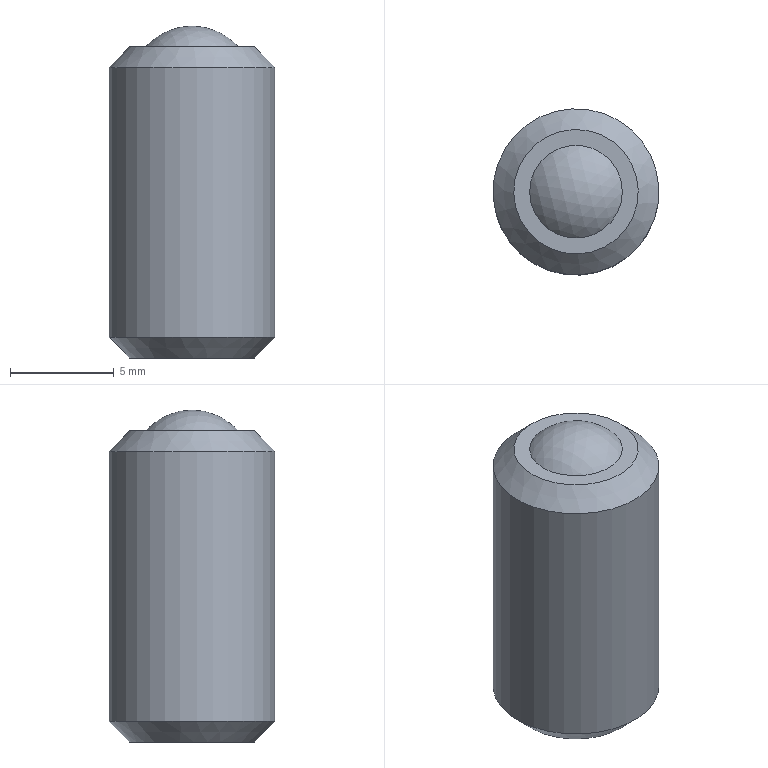Part | STEP file | 车灯-后视镜_id346_x_t | 1 solid | 6 faces | box 8 x 8 x 16 mm | volume 739.323 mm3 | plane 2 | cone 2 | cylinder 1 | sphere 1 | commonest cylinder face diameters 8 x1
STEP:
#1=CARTESIAN_POINT('',(-108.175,-125.605,-25.147));
#2=VERTEX_POINT('',#1);
#3=CARTESIAN_POINT('',(-105.27,-124.855,-25.147));
#4=DIRECTION('',(0.,0.,1.));
#5=DIRECTION('',(-0.9683,-0.2498,0.));
#6=AXIS2_PLACEMENT_3D('',#3,#4,#5);
#7=CIRCLE('',#6,3.);
#8=EDGE_CURVE('',#2,#2,#7,.T.);
#9=ORIENTED_EDGE('',*,*,#8,.T.);
#10=EDGE_LOOP('',(#9));
#11=FACE_BOUND('',#10,.T.);
#12=CARTESIAN_POINT('',(-107.435,-125.414,-25.147));
#13=VERTEX_POINT('',#12);
#14=CARTESIAN_POINT('',(-105.27,-124.855,-25.147));
#15=DIRECTION('',(0.,0.,1.));
#16=DIRECTION('',(-0.9683,-0.2498,0.));
#17=AXIS2_PLACEMENT_3D('',#14,#15,#16);
#18=CIRCLE('',#17,2.236);
#19=EDGE_CURVE('',#13,#13,#18,.T.);
#20=ORIENTED_EDGE('',*,*,#19,.F.);
#21=EDGE_LOOP('',(#20));
#22=FACE_BOUND('',#21,.T.);
#23=CARTESIAN_POINT('',(-105.27,-124.855,-25.147));
#24=DIRECTION('',(0.,0.,1.));
#25=DIRECTION('',(-0.9683,-0.2498,0.));
#26=AXIS2_PLACEMENT_3D('',#23,#24,#25);
#27=PLANE('',#26);
#28=ADVANCED_FACE('',(#11,#22),#27,.T.);
#29=CARTESIAN_POINT('',(-102.365,-124.106,-40.147));
#30=VERTEX_POINT('',#29);
#31=CARTESIAN_POINT('',(-105.27,-124.855,-40.147));
#32=DIRECTION('',(0.,0.,-1.));
#33=DIRECTION('',(0.9683,0.2498,0.));
#34=AXIS2_PLACEMENT_3D('',#31,#32,#33);
#35=CIRCLE('',#34,3.);
#36=EDGE_CURVE('',#30,#30,#35,.T.);
#37=ORIENTED_EDGE('',*,*,#36,.T.);
#38=EDGE_LOOP('',(#37));
#39=FACE_OUTER_BOUND('',#38,.T.);
#40=CARTESIAN_POINT('',(-105.27,-124.855,-40.147));
#41=DIRECTION('',(0.,0.,-1.));
#42=DIRECTION('',(0.9683,0.2498,0.));
#43=AXIS2_PLACEMENT_3D('',#40,#41,#42);
#44=PLANE('',#43);
#45=ADVANCED_FACE('',(#39),#44,.T.);
#46=CARTESIAN_POINT('',(-101.397,-123.856,-39.147));
#47=VERTEX_POINT('',#46);
#48=CARTESIAN_POINT('',(-105.27,-124.855,-39.147));
#49=DIRECTION('',(0.,0.,1.));
#50=DIRECTION('',(0.9683,0.2498,0.));
#51=AXIS2_PLACEMENT_3D('',#48,#49,#50);
#52=CIRCLE('',#51,4.);
#53=EDGE_CURVE('',#47,#47,#52,.T.);
#54=ORIENTED_EDGE('',*,*,#53,.T.);
#55=EDGE_LOOP('',(#54));
#56=FACE_BOUND('',#55,.T.);
#57=CARTESIAN_POINT('',(-109.143,-125.854,-26.147));
#58=VERTEX_POINT('',#57);
#59=CARTESIAN_POINT('',(-105.27,-124.855,-26.147));
#60=DIRECTION('',(0.,0.,-1.));
#61=DIRECTION('',(-0.9683,-0.2498,0.));
#62=AXIS2_PLACEMENT_3D('',#59,#60,#61);
#63=CIRCLE('',#62,4.);
#64=EDGE_CURVE('',#58,#58,#63,.T.);
#65=ORIENTED_EDGE('',*,*,#64,.T.);
#66=EDGE_LOOP('',(#65));
#67=FACE_BOUND('',#66,.T.);
#68=CARTESIAN_POINT('',(-105.27,-124.855,-40.147));
#69=DIRECTION('',(0.,0.,1.));
#70=DIRECTION('',(-0.9683,-0.2498,0.));
#71=AXIS2_PLACEMENT_3D('',#68,#69,#70);
#72=CYLINDRICAL_SURFACE('',#71,4.);
#73=ADVANCED_FACE('',(#56,#67),#72,.T.);
#74=ORIENTED_EDGE('',*,*,#19,.T.);
#75=EDGE_LOOP('',(#74));
#76=FACE_OUTER_BOUND('',#75,.T.);
#77=CARTESIAN_POINT('',(-105.27,-124.855,-27.147));
#78=DIRECTION('',(-0.9683,-0.2498,0.));
#79=DIRECTION('',(-0.2498,0.9683,0.));
#80=AXIS2_PLACEMENT_3D('',#77,#78,#79);
#81=SPHERICAL_SURFACE('',#80,3.);
#82=ADVANCED_FACE('',(#76),#81,.T.);
#83=ORIENTED_EDGE('',*,*,#53,.F.);
#84=EDGE_LOOP('',(#83));
#85=FACE_BOUND('',#84,.T.);
#86=ORIENTED_EDGE('',*,*,#36,.F.);
#87=EDGE_LOOP('',(#86));
#88=FACE_BOUND('',#87,.T.);
#89=CARTESIAN_POINT('',(-105.27,-124.855,-40.147));
#90=DIRECTION('',(0.,0.,1.));
#91=DIRECTION('',(-0.9683,-0.2498,0.));
#92=AXIS2_PLACEMENT_3D('',#89,#90,#91);
#93=CONICAL_SURFACE('',#92,3.,45.);
#94=ADVANCED_FACE('',(#85,#88),#93,.T.);
#95=ORIENTED_EDGE('',*,*,#64,.F.);
#96=EDGE_LOOP('',(#95));
#97=FACE_BOUND('',#96,.T.);
#98=ORIENTED_EDGE('',*,*,#8,.F.);
#99=EDGE_LOOP('',(#98));
#100=FACE_BOUND('',#99,.T.);
#101=CARTESIAN_POINT('',(-105.27,-124.855,-25.147));
#102=DIRECTION('',(0.,0.,-1.));
#103=DIRECTION('',(0.9683,0.2498,0.));
#104=AXIS2_PLACEMENT_3D('',#101,#102,#103);
#105=CONICAL_SURFACE('',#104,3.,45.);
#106=ADVANCED_FACE('',(#97,#100),#105,.T.);
#107=CLOSED_SHELL('',(#28,#45,#73,#82,#94,#106));
#108=MANIFOLD_SOLID_BREP('',#107);
#109=(LENGTH_UNIT()NAMED_UNIT(*)SI_UNIT(.MILLI.,.METRE.));
#110=UNCERTAINTY_MEASURE_WITH_UNIT(LENGTH_MEASURE(0.00002),#109,'','');
#111=(NAMED_UNIT(*)PLANE_ANGLE_UNIT()SI_UNIT($,.RADIAN.));
#112=PLANE_ANGLE_MEASURE_WITH_UNIT(PLANE_ANGLE_MEASURE(0.01745),#111);
#113=DIMENSIONAL_EXPONENTS(0.,0.,0.,0.,0.,0.,0.);
#114=(CONVERSION_BASED_UNIT('DEGREE',#112)NAMED_UNIT(#113)PLANE_ANGLE_UNIT());
#115=(NAMED_UNIT(*)SI_UNIT($,.STERADIAN.)SOLID_ANGLE_UNIT());
#116=(GEOMETRIC_REPRESENTATION_CONTEXT(3)GLOBAL_UNCERTAINTY_ASSIGNED_CONTEXT((#110))GLOBAL_UNIT_ASSIGNED_CONTEXT((#109,#114,#115))REPRESENTATION_CONTEXT('',''));
#117=ADVANCED_BREP_SHAPE_REPRESENTATION('',(#108),#116);